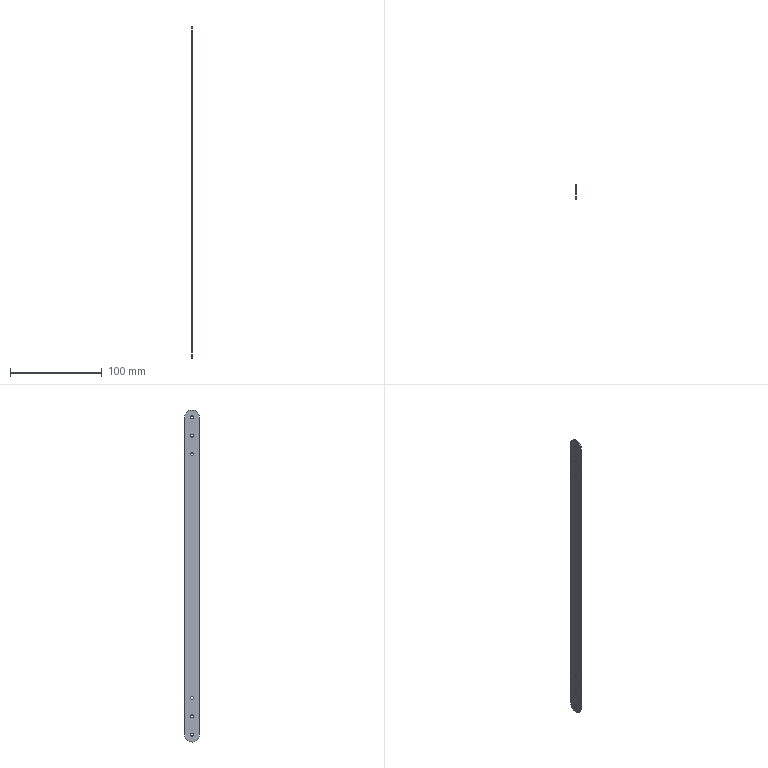Part | SolidWorks | features BaseBody 1 | 1 solid | 19 faces | box 1 x 16 x 361 mm | volume 5673 mm3 | cylinder 15 | plane 4 | commonest cylinder face diameters 3.2 x12 16 x3
STEP:
#1=CARTESIAN_POINT('',(1.,0.,-232.464));
#2=VERTEX_POINT('',#1);
#3=CARTESIAN_POINT('',(1.,0.,-235.664));
#4=VERTEX_POINT('',#3);
#5=CARTESIAN_POINT('',(1.,0.,-234.064));
#6=DIRECTION('',(1.,0.,0.));
#7=DIRECTION('',(0.,0.,1.));
#8=AXIS2_PLACEMENT_3D('',#5,#6,#7);
#9=CIRCLE('',#8,1.6);
#10=EDGE_CURVE('',#2,#4,#9,.T.);
#11=ORIENTED_EDGE('',*,*,#10,.T.);
#12=CARTESIAN_POINT('',(0.,0.,-235.664));
#13=VERTEX_POINT('',#12);
#14=CARTESIAN_POINT('',(1.,0.,-235.664));
#15=DIRECTION('',(-1.,0.,0.));
#16=VECTOR('',#15,1000.);
#17=LINE('',#14,#16);
#18=EDGE_CURVE('',#4,#13,#17,.T.);
#19=ORIENTED_EDGE('',*,*,#18,.T.);
#20=CARTESIAN_POINT('',(0.,0.,-232.464));
#21=VERTEX_POINT('',#20);
#22=CARTESIAN_POINT('',(0.,0.,-234.064));
#23=DIRECTION('',(-1.,0.,0.));
#24=DIRECTION('',(0.,0.,1.));
#25=AXIS2_PLACEMENT_3D('',#22,#23,#24);
#26=CIRCLE('',#25,1.6);
#27=EDGE_CURVE('',#13,#21,#26,.T.);
#28=ORIENTED_EDGE('',*,*,#27,.T.);
#29=CARTESIAN_POINT('',(1.,0.,-232.464));
#30=DIRECTION('',(-1.,0.,0.));
#31=VECTOR('',#30,1000.);
#32=LINE('',#29,#31);
#33=EDGE_CURVE('',#2,#21,#32,.T.);
#34=ORIENTED_EDGE('',*,*,#33,.F.);
#35=EDGE_LOOP('',(#11,#19,#28,#34));
#36=FACE_OUTER_BOUND('',#35,.T.);
#37=CARTESIAN_POINT('',(1.,0.,-234.064));
#38=DIRECTION('',(-1.,0.,0.));
#39=DIRECTION('',(0.,0.,1.));
#40=AXIS2_PLACEMENT_3D('',#37,#38,#39);
#41=CYLINDRICAL_SURFACE('',#40,1.6);
#42=ADVANCED_FACE('',(#36),#41,.F.);
#43=CARTESIAN_POINT('',(1.,0.,-275.664));
#44=VERTEX_POINT('',#43);
#45=CARTESIAN_POINT('',(1.,0.,-272.464));
#46=VERTEX_POINT('',#45);
#47=CARTESIAN_POINT('',(1.,0.,-274.064));
#48=DIRECTION('',(-1.,0.,0.));
#49=DIRECTION('',(0.,0.,1.));
#50=AXIS2_PLACEMENT_3D('',#47,#48,#49);
#51=CIRCLE('',#50,1.6);
#52=EDGE_CURVE('',#44,#46,#51,.T.);
#53=ORIENTED_EDGE('',*,*,#52,.F.);
#54=CARTESIAN_POINT('',(0.,0.,-275.664));
#55=VERTEX_POINT('',#54);
#56=CARTESIAN_POINT('',(1.,0.,-275.664));
#57=DIRECTION('',(-1.,0.,0.));
#58=VECTOR('',#57,1000.);
#59=LINE('',#56,#58);
#60=EDGE_CURVE('',#44,#55,#59,.T.);
#61=ORIENTED_EDGE('',*,*,#60,.T.);
#62=CARTESIAN_POINT('',(0.,0.,-272.464));
#63=VERTEX_POINT('',#62);
#64=CARTESIAN_POINT('',(0.,0.,-274.064));
#65=DIRECTION('',(-1.,0.,0.));
#66=DIRECTION('',(0.,0.,1.));
#67=AXIS2_PLACEMENT_3D('',#64,#65,#66);
#68=CIRCLE('',#67,1.6);
#69=EDGE_CURVE('',#55,#63,#68,.T.);
#70=ORIENTED_EDGE('',*,*,#69,.T.);
#71=CARTESIAN_POINT('',(1.,0.,-272.464));
#72=DIRECTION('',(-1.,0.,0.));
#73=VECTOR('',#72,1000.);
#74=LINE('',#71,#73);
#75=EDGE_CURVE('',#46,#63,#74,.T.);
#76=ORIENTED_EDGE('',*,*,#75,.F.);
#77=EDGE_LOOP('',(#53,#61,#70,#76));
#78=FACE_OUTER_BOUND('',#77,.T.);
#79=CARTESIAN_POINT('',(1.,0.,-274.064));
#80=DIRECTION('',(-1.,0.,0.));
#81=DIRECTION('',(0.,0.,1.));
#82=AXIS2_PLACEMENT_3D('',#79,#80,#81);
#83=CYLINDRICAL_SURFACE('',#82,1.6);
#84=ADVANCED_FACE('',(#78),#83,.F.);
#85=CARTESIAN_POINT('',(1.,0.,49.336));
#86=VERTEX_POINT('',#85);
#87=CARTESIAN_POINT('',(1.,0.,52.536));
#88=VERTEX_POINT('',#87);
#89=CARTESIAN_POINT('',(1.,0.,50.936));
#90=DIRECTION('',(-1.,0.,0.));
#91=DIRECTION('',(0.,0.,1.));
#92=AXIS2_PLACEMENT_3D('',#89,#90,#91);
#93=CIRCLE('',#92,1.6);
#94=EDGE_CURVE('',#86,#88,#93,.T.);
#95=ORIENTED_EDGE('',*,*,#94,.F.);
#96=CARTESIAN_POINT('',(0.,0.,49.336));
#97=VERTEX_POINT('',#96);
#98=CARTESIAN_POINT('',(1.,0.,49.336));
#99=DIRECTION('',(-1.,0.,0.));
#100=VECTOR('',#99,1000.);
#101=LINE('',#98,#100);
#102=EDGE_CURVE('',#86,#97,#101,.T.);
#103=ORIENTED_EDGE('',*,*,#102,.T.);
#104=CARTESIAN_POINT('',(0.,0.,52.536));
#105=VERTEX_POINT('',#104);
#106=CARTESIAN_POINT('',(0.,0.,50.936));
#107=DIRECTION('',(-1.,0.,0.));
#108=DIRECTION('',(0.,0.,1.));
#109=AXIS2_PLACEMENT_3D('',#106,#107,#108);
#110=CIRCLE('',#109,1.6);
#111=EDGE_CURVE('',#97,#105,#110,.T.);
#112=ORIENTED_EDGE('',*,*,#111,.T.);
#113=CARTESIAN_POINT('',(1.,0.,52.536));
#114=DIRECTION('',(-1.,0.,0.));
#115=VECTOR('',#114,1000.);
#116=LINE('',#113,#115);
#117=EDGE_CURVE('',#88,#105,#116,.T.);
#118=ORIENTED_EDGE('',*,*,#117,.F.);
#119=EDGE_LOOP('',(#95,#103,#112,#118));
#120=FACE_OUTER_BOUND('',#119,.T.);
#121=CARTESIAN_POINT('',(1.,0.,50.936));
#122=DIRECTION('',(-1.,0.,0.));
#123=DIRECTION('',(0.,0.,1.));
#124=AXIS2_PLACEMENT_3D('',#121,#122,#123);
#125=CYLINDRICAL_SURFACE('',#124,1.6);
#126=ADVANCED_FACE('',(#120),#125,.F.);
#127=CARTESIAN_POINT('',(1.,0.,69.336));
#128=VERTEX_POINT('',#127);
#129=CARTESIAN_POINT('',(1.,0.,72.536));
#130=VERTEX_POINT('',#129);
#131=CARTESIAN_POINT('',(1.,0.,70.936));
#132=DIRECTION('',(-1.,0.,0.));
#133=DIRECTION('',(0.,0.,1.));
#134=AXIS2_PLACEMENT_3D('',#131,#132,#133);
#135=CIRCLE('',#134,1.6);
#136=EDGE_CURVE('',#128,#130,#135,.T.);
#137=ORIENTED_EDGE('',*,*,#136,.F.);
#138=CARTESIAN_POINT('',(0.,0.,69.336));
#139=VERTEX_POINT('',#138);
#140=CARTESIAN_POINT('',(1.,0.,69.336));
#141=DIRECTION('',(-1.,0.,0.));
#142=VECTOR('',#141,1000.);
#143=LINE('',#140,#142);
#144=EDGE_CURVE('',#128,#139,#143,.T.);
#145=ORIENTED_EDGE('',*,*,#144,.T.);
#146=CARTESIAN_POINT('',(0.,0.,72.536));
#147=VERTEX_POINT('',#146);
#148=CARTESIAN_POINT('',(0.,0.,70.936));
#149=DIRECTION('',(-1.,0.,0.));
#150=DIRECTION('',(0.,0.,1.));
#151=AXIS2_PLACEMENT_3D('',#148,#149,#150);
#152=CIRCLE('',#151,1.6);
#153=EDGE_CURVE('',#139,#147,#152,.T.);
#154=ORIENTED_EDGE('',*,*,#153,.T.);
#155=CARTESIAN_POINT('',(1.,0.,72.536));
#156=DIRECTION('',(-1.,0.,0.));
#157=VECTOR('',#156,1000.);
#158=LINE('',#155,#157);
#159=EDGE_CURVE('',#130,#147,#158,.T.);
#160=ORIENTED_EDGE('',*,*,#159,.F.);
#161=EDGE_LOOP('',(#137,#145,#154,#160));
#162=FACE_OUTER_BOUND('',#161,.T.);
#163=CARTESIAN_POINT('',(1.,0.,70.936));
#164=DIRECTION('',(-1.,0.,0.));
#165=DIRECTION('',(0.,0.,1.));
#166=AXIS2_PLACEMENT_3D('',#163,#164,#165);
#167=CYLINDRICAL_SURFACE('',#166,1.6);
#168=ADVANCED_FACE('',(#162),#167,.F.);
#169=CARTESIAN_POINT('',(1.,0.,29.336));
#170=VERTEX_POINT('',#169);
#171=CARTESIAN_POINT('',(1.,0.,32.536));
#172=VERTEX_POINT('',#171);
#173=CARTESIAN_POINT('',(1.,0.,30.936));
#174=DIRECTION('',(-1.,0.,0.));
#175=DIRECTION('',(0.,0.,1.));
#176=AXIS2_PLACEMENT_3D('',#173,#174,#175);
#177=CIRCLE('',#176,1.6);
#178=EDGE_CURVE('',#170,#172,#177,.T.);
#179=ORIENTED_EDGE('',*,*,#178,.F.);
#180=CARTESIAN_POINT('',(0.,0.,29.336));
#181=VERTEX_POINT('',#180);
#182=CARTESIAN_POINT('',(1.,0.,29.336));
#183=DIRECTION('',(-1.,0.,0.));
#184=VECTOR('',#183,1000.);
#185=LINE('',#182,#184);
#186=EDGE_CURVE('',#170,#181,#185,.T.);
#187=ORIENTED_EDGE('',*,*,#186,.T.);
#188=CARTESIAN_POINT('',(0.,0.,32.536));
#189=VERTEX_POINT('',#188);
#190=CARTESIAN_POINT('',(0.,0.,30.936));
#191=DIRECTION('',(-1.,0.,0.));
#192=DIRECTION('',(0.,0.,1.));
#193=AXIS2_PLACEMENT_3D('',#190,#191,#192);
#194=CIRCLE('',#193,1.6);
#195=EDGE_CURVE('',#181,#189,#194,.T.);
#196=ORIENTED_EDGE('',*,*,#195,.T.);
#197=CARTESIAN_POINT('',(1.,0.,32.536));
#198=DIRECTION('',(-1.,0.,0.));
#199=VECTOR('',#198,1000.);
#200=LINE('',#197,#199);
#201=EDGE_CURVE('',#172,#189,#200,.T.);
#202=ORIENTED_EDGE('',*,*,#201,.F.);
#203=EDGE_LOOP('',(#179,#187,#196,#202));
#204=FACE_OUTER_BOUND('',#203,.T.);
#205=CARTESIAN_POINT('',(1.,0.,30.936));
#206=DIRECTION('',(-1.,0.,0.));
#207=DIRECTION('',(0.,0.,1.));
#208=AXIS2_PLACEMENT_3D('',#205,#206,#207);
#209=CYLINDRICAL_SURFACE('',#208,1.6);
#210=ADVANCED_FACE('',(#204),#209,.F.);
#211=CARTESIAN_POINT('',(1.,0.,-255.664));
#212=VERTEX_POINT('',#211);
#213=CARTESIAN_POINT('',(1.,0.,-252.464));
#214=VERTEX_POINT('',#213);
#215=CARTESIAN_POINT('',(1.,0.,-254.064));
#216=DIRECTION('',(-1.,0.,0.));
#217=DIRECTION('',(0.,0.,1.));
#218=AXIS2_PLACEMENT_3D('',#215,#216,#217);
#219=CIRCLE('',#218,1.6);
#220=EDGE_CURVE('',#212,#214,#219,.T.);
#221=ORIENTED_EDGE('',*,*,#220,.F.);
#222=CARTESIAN_POINT('',(0.,0.,-255.664));
#223=VERTEX_POINT('',#222);
#224=CARTESIAN_POINT('',(1.,0.,-255.664));
#225=DIRECTION('',(-1.,0.,0.));
#226=VECTOR('',#225,1000.);
#227=LINE('',#224,#226);
#228=EDGE_CURVE('',#212,#223,#227,.T.);
#229=ORIENTED_EDGE('',*,*,#228,.T.);
#230=CARTESIAN_POINT('',(0.,0.,-252.464));
#231=VERTEX_POINT('',#230);
#232=CARTESIAN_POINT('',(0.,0.,-254.064));
#233=DIRECTION('',(-1.,0.,0.));
#234=DIRECTION('',(0.,0.,1.));
#235=AXIS2_PLACEMENT_3D('',#232,#233,#234);
#236=CIRCLE('',#235,1.6);
#237=EDGE_CURVE('',#223,#231,#236,.T.);
#238=ORIENTED_EDGE('',*,*,#237,.T.);
#239=CARTESIAN_POINT('',(1.,0.,-252.464));
#240=DIRECTION('',(-1.,0.,0.));
#241=VECTOR('',#240,1000.);
#242=LINE('',#239,#241);
#243=EDGE_CURVE('',#214,#231,#242,.T.);
#244=ORIENTED_EDGE('',*,*,#243,.F.);
#245=EDGE_LOOP('',(#221,#229,#238,#244));
#246=FACE_OUTER_BOUND('',#245,.T.);
#247=CARTESIAN_POINT('',(1.,0.,-254.064));
#248=DIRECTION('',(-1.,0.,0.));
#249=DIRECTION('',(0.,0.,1.));
#250=AXIS2_PLACEMENT_3D('',#247,#248,#249);
#251=CYLINDRICAL_SURFACE('',#250,1.6);
#252=ADVANCED_FACE('',(#246),#251,.F.);
#253=CARTESIAN_POINT('',(1.,0.,78.936));
#254=VERTEX_POINT('',#253);
#255=CARTESIAN_POINT('',(1.,-8.,70.936));
#256=VERTEX_POINT('',#255);
#257=CARTESIAN_POINT('',(1.,0.,70.936));
#258=DIRECTION('',(1.,0.,0.));
#259=DIRECTION('',(0.,0.,1.));
#260=AXIS2_PLACEMENT_3D('',#257,#258,#259);
#261=CIRCLE('',#260,8.);
#262=EDGE_CURVE('',#254,#256,#261,.T.);
#263=ORIENTED_EDGE('',*,*,#262,.F.);
#264=CARTESIAN_POINT('',(0.,0.,78.936));
#265=VERTEX_POINT('',#264);
#266=CARTESIAN_POINT('',(1.,0.,78.936));
#267=DIRECTION('',(-1.,0.,0.));
#268=VECTOR('',#267,1000.);
#269=LINE('',#266,#268);
#270=EDGE_CURVE('',#254,#265,#269,.T.);
#271=ORIENTED_EDGE('',*,*,#270,.T.);
#272=CARTESIAN_POINT('',(0.,-8.,70.936));
#273=VERTEX_POINT('',#272);
#274=CARTESIAN_POINT('',(0.,0.,70.936));
#275=DIRECTION('',(1.,0.,0.));
#276=DIRECTION('',(0.,0.,1.));
#277=AXIS2_PLACEMENT_3D('',#274,#275,#276);
#278=CIRCLE('',#277,8.);
#279=EDGE_CURVE('',#265,#273,#278,.T.);
#280=ORIENTED_EDGE('',*,*,#279,.T.);
#281=CARTESIAN_POINT('',(0.5,-8.,70.936));
#282=DIRECTION('',(1.,0.,0.));
#283=VECTOR('',#282,1000.);
#284=LINE('',#281,#283);
#285=EDGE_CURVE('',#273,#256,#284,.T.);
#286=ORIENTED_EDGE('',*,*,#285,.T.);
#287=EDGE_LOOP('',(#263,#271,#280,#286));
#288=FACE_OUTER_BOUND('',#287,.T.);
#289=CARTESIAN_POINT('',(1.,0.,70.936));
#290=DIRECTION('',(-1.,0.,0.));
#291=DIRECTION('',(0.,0.,1.));
#292=AXIS2_PLACEMENT_3D('',#289,#290,#291);
#293=CYLINDRICAL_SURFACE('',#292,8.);
#294=ADVANCED_FACE('',(#288),#293,.T.);
#295=ORIENTED_EDGE('',*,*,#18,.F.);
#296=CARTESIAN_POINT('',(1.,0.,-234.064));
#297=DIRECTION('',(1.,0.,0.));
#298=DIRECTION('',(0.,0.,1.));
#299=AXIS2_PLACEMENT_3D('',#296,#297,#298);
#300=CIRCLE('',#299,1.6);
#301=EDGE_CURVE('',#4,#2,#300,.T.);
#302=ORIENTED_EDGE('',*,*,#301,.T.);
#303=ORIENTED_EDGE('',*,*,#33,.T.);
#304=CARTESIAN_POINT('',(0.,0.,-234.064));
#305=DIRECTION('',(-1.,0.,0.));
#306=DIRECTION('',(0.,0.,1.));
#307=AXIS2_PLACEMENT_3D('',#304,#305,#306);
#308=CIRCLE('',#307,1.6);
#309=EDGE_CURVE('',#21,#13,#308,.T.);
#310=ORIENTED_EDGE('',*,*,#309,.T.);
#311=EDGE_LOOP('',(#295,#302,#303,#310));
#312=FACE_OUTER_BOUND('',#311,.T.);
#313=CARTESIAN_POINT('',(1.,0.,-234.064));
#314=DIRECTION('',(-1.,0.,0.));
#315=DIRECTION('',(0.,0.,1.));
#316=AXIS2_PLACEMENT_3D('',#313,#314,#315);
#317=CYLINDRICAL_SURFACE('',#316,1.6);
#318=ADVANCED_FACE('',(#312),#317,.F.);
#319=ORIENTED_EDGE('',*,*,#309,.F.);
#320=ORIENTED_EDGE('',*,*,#27,.F.);
#321=EDGE_LOOP('',(#319,#320));
#322=FACE_BOUND('',#321,.T.);
#323=CARTESIAN_POINT('',(0.,0.,-274.064));
#324=DIRECTION('',(-1.,0.,0.));
#325=DIRECTION('',(0.,0.,1.));
#326=AXIS2_PLACEMENT_3D('',#323,#324,#325);
#327=CIRCLE('',#326,1.6);
#328=EDGE_CURVE('',#63,#55,#327,.T.);
#329=ORIENTED_EDGE('',*,*,#328,.F.);
#330=ORIENTED_EDGE('',*,*,#69,.F.);
#331=EDGE_LOOP('',(#329,#330));
#332=FACE_BOUND('',#331,.T.);
#333=CARTESIAN_POINT('',(0.,0.,50.936));
#334=DIRECTION('',(-1.,0.,0.));
#335=DIRECTION('',(0.,0.,1.));
#336=AXIS2_PLACEMENT_3D('',#333,#334,#335);
#337=CIRCLE('',#336,1.6);
#338=EDGE_CURVE('',#105,#97,#337,.T.);
#339=ORIENTED_EDGE('',*,*,#338,.F.);
#340=ORIENTED_EDGE('',*,*,#111,.F.);
#341=EDGE_LOOP('',(#339,#340));
#342=FACE_BOUND('',#341,.T.);
#343=CARTESIAN_POINT('',(0.,0.,70.936));
#344=DIRECTION('',(-1.,0.,0.));
#345=DIRECTION('',(0.,0.,1.));
#346=AXIS2_PLACEMENT_3D('',#343,#344,#345);
#347=CIRCLE('',#346,1.6);
#348=EDGE_CURVE('',#147,#139,#347,.T.);
#349=ORIENTED_EDGE('',*,*,#348,.F.);
#350=ORIENTED_EDGE('',*,*,#153,.F.);
#351=EDGE_LOOP('',(#349,#350));
#352=FACE_BOUND('',#351,.T.);
#353=CARTESIAN_POINT('',(0.,0.,30.936));
#354=DIRECTION('',(-1.,0.,0.));
#355=DIRECTION('',(0.,0.,1.));
#356=AXIS2_PLACEMENT_3D('',#353,#354,#355);
#357=CIRCLE('',#356,1.6);
#358=EDGE_CURVE('',#189,#181,#357,.T.);
#359=ORIENTED_EDGE('',*,*,#358,.F.);
#360=ORIENTED_EDGE('',*,*,#195,.F.);
#361=EDGE_LOOP('',(#359,#360));
#362=FACE_BOUND('',#361,.T.);
#363=CARTESIAN_POINT('',(0.,0.,-254.064));
#364=DIRECTION('',(-1.,0.,0.));
#365=DIRECTION('',(0.,0.,1.));
#366=AXIS2_PLACEMENT_3D('',#363,#364,#365);
#367=CIRCLE('',#366,1.6);
#368=EDGE_CURVE('',#231,#223,#367,.T.);
#369=ORIENTED_EDGE('',*,*,#368,.F.);
#370=ORIENTED_EDGE('',*,*,#237,.F.);
#371=EDGE_LOOP('',(#369,#370));
#372=FACE_BOUND('',#371,.T.);
#373=CARTESIAN_POINT('',(0.,8.,-274.064));
#374=VERTEX_POINT('',#373);
#375=CARTESIAN_POINT('',(0.,8.,70.936));
#376=VERTEX_POINT('',#375);
#377=CARTESIAN_POINT('',(0.,8.,-101.564));
#378=DIRECTION('',(0.,0.,1.));
#379=VECTOR('',#378,1000.);
#380=LINE('',#377,#379);
#381=EDGE_CURVE('',#374,#376,#380,.T.);
#382=ORIENTED_EDGE('',*,*,#381,.F.);
#383=CARTESIAN_POINT('',(0.,-8.,-274.064));
#384=VERTEX_POINT('',#383);
#385=CARTESIAN_POINT('',(0.,0.,-274.064));
#386=DIRECTION('',(1.,0.,0.));
#387=DIRECTION('',(0.,0.,1.));
#388=AXIS2_PLACEMENT_3D('',#385,#386,#387);
#389=CIRCLE('',#388,8.);
#390=EDGE_CURVE('',#384,#374,#389,.T.);
#391=ORIENTED_EDGE('',*,*,#390,.F.);
#392=CARTESIAN_POINT('',(0.,-8.,-101.564));
#393=DIRECTION('',(0.,0.,-1.));
#394=VECTOR('',#393,1000.);
#395=LINE('',#392,#394);
#396=EDGE_CURVE('',#273,#384,#395,.T.);
#397=ORIENTED_EDGE('',*,*,#396,.F.);
#398=ORIENTED_EDGE('',*,*,#279,.F.);
#399=CARTESIAN_POINT('',(0.,0.,70.936));
#400=DIRECTION('',(1.,0.,0.));
#401=DIRECTION('',(0.,0.,1.));
#402=AXIS2_PLACEMENT_3D('',#399,#400,#401);
#403=CIRCLE('',#402,8.);
#404=EDGE_CURVE('',#376,#265,#403,.T.);
#405=ORIENTED_EDGE('',*,*,#404,.F.);
#406=EDGE_LOOP('',(#382,#391,#397,#398,#405));
#407=FACE_OUTER_BOUND('',#406,.T.);
#408=CARTESIAN_POINT('',(0.,-8.,81.102));
#409=DIRECTION('',(1.,0.,0.));
#410=DIRECTION('',(0.,0.,-1.));
#411=AXIS2_PLACEMENT_3D('',#408,#409,#410);
#412=PLANE('',#411);
#413=ADVANCED_FACE('',(#322,#332,#342,#352,#362,#372,#407),#412,.F.);
#414=ORIENTED_EDGE('',*,*,#10,.F.);
#415=ORIENTED_EDGE('',*,*,#301,.F.);
#416=EDGE_LOOP('',(#414,#415));
#417=FACE_BOUND('',#416,.T.);
#418=CARTESIAN_POINT('',(1.,0.,-274.064));
#419=DIRECTION('',(-1.,0.,0.));
#420=DIRECTION('',(0.,0.,1.));
#421=AXIS2_PLACEMENT_3D('',#418,#419,#420);
#422=CIRCLE('',#421,1.6);
#423=EDGE_CURVE('',#46,#44,#422,.T.);
#424=ORIENTED_EDGE('',*,*,#423,.T.);
#425=ORIENTED_EDGE('',*,*,#52,.T.);
#426=EDGE_LOOP('',(#424,#425));
#427=FACE_BOUND('',#426,.T.);
#428=CARTESIAN_POINT('',(1.,0.,50.936));
#429=DIRECTION('',(-1.,0.,0.));
#430=DIRECTION('',(0.,0.,1.));
#431=AXIS2_PLACEMENT_3D('',#428,#429,#430);
#432=CIRCLE('',#431,1.6);
#433=EDGE_CURVE('',#88,#86,#432,.T.);
#434=ORIENTED_EDGE('',*,*,#433,.T.);
#435=ORIENTED_EDGE('',*,*,#94,.T.);
#436=EDGE_LOOP('',(#434,#435));
#437=FACE_BOUND('',#436,.T.);
#438=CARTESIAN_POINT('',(1.,0.,70.936));
#439=DIRECTION('',(-1.,0.,0.));
#440=DIRECTION('',(0.,0.,1.));
#441=AXIS2_PLACEMENT_3D('',#438,#439,#440);
#442=CIRCLE('',#441,1.6);
#443=EDGE_CURVE('',#130,#128,#442,.T.);
#444=ORIENTED_EDGE('',*,*,#443,.T.);
#445=ORIENTED_EDGE('',*,*,#136,.T.);
#446=EDGE_LOOP('',(#444,#445));
#447=FACE_BOUND('',#446,.T.);
#448=CARTESIAN_POINT('',(1.,0.,30.936));
#449=DIRECTION('',(-1.,0.,0.));
#450=DIRECTION('',(0.,0.,1.));
#451=AXIS2_PLACEMENT_3D('',#448,#449,#450);
#452=CIRCLE('',#451,1.6);
#453=EDGE_CURVE('',#172,#170,#452,.T.);
#454=ORIENTED_EDGE('',*,*,#453,.T.);
#455=ORIENTED_EDGE('',*,*,#178,.T.);
#456=EDGE_LOOP('',(#454,#455));
#457=FACE_BOUND('',#456,.T.);
#458=CARTESIAN_POINT('',(1.,0.,-254.064));
#459=DIRECTION('',(-1.,0.,0.));
#460=DIRECTION('',(0.,0.,1.));
#461=AXIS2_PLACEMENT_3D('',#458,#459,#460);
#462=CIRCLE('',#461,1.6);
#463=EDGE_CURVE('',#214,#212,#462,.T.);
#464=ORIENTED_EDGE('',*,*,#463,.T.);
#465=ORIENTED_EDGE('',*,*,#220,.T.);
#466=EDGE_LOOP('',(#464,#465));
#467=FACE_BOUND('',#466,.T.);
#468=CARTESIAN_POINT('',(1.,-8.,-274.064));
#469=VERTEX_POINT('',#468);
#470=CARTESIAN_POINT('',(1.,8.,-274.064));
#471=VERTEX_POINT('',#470);
#472=CARTESIAN_POINT('',(1.,0.,-274.064));
#473=DIRECTION('',(1.,0.,0.));
#474=DIRECTION('',(0.,0.,1.));
#475=AXIS2_PLACEMENT_3D('',#472,#473,#474);
#476=CIRCLE('',#475,8.);
#477=EDGE_CURVE('',#469,#471,#476,.T.);
#478=ORIENTED_EDGE('',*,*,#477,.T.);
#479=CARTESIAN_POINT('',(1.,8.,70.936));
#480=VERTEX_POINT('',#479);
#481=CARTESIAN_POINT('',(1.,8.,-101.564));
#482=DIRECTION('',(0.,0.,1.));
#483=VECTOR('',#482,1000.);
#484=LINE('',#481,#483);
#485=EDGE_CURVE('',#471,#480,#484,.T.);
#486=ORIENTED_EDGE('',*,*,#485,.T.);
#487=CARTESIAN_POINT('',(1.,0.,70.936));
#488=DIRECTION('',(1.,0.,0.));
#489=DIRECTION('',(0.,0.,1.));
#490=AXIS2_PLACEMENT_3D('',#487,#488,#489);
#491=CIRCLE('',#490,8.);
#492=EDGE_CURVE('',#480,#254,#491,.T.);
#493=ORIENTED_EDGE('',*,*,#492,.T.);
#494=ORIENTED_EDGE('',*,*,#262,.T.);
#495=CARTESIAN_POINT('',(1.,-8.,-101.564));
#496=DIRECTION('',(0.,0.,-1.));
#497=VECTOR('',#496,1000.);
#498=LINE('',#495,#497);
#499=EDGE_CURVE('',#256,#469,#498,.T.);
#500=ORIENTED_EDGE('',*,*,#499,.T.);
#501=EDGE_LOOP('',(#478,#486,#493,#494,#500));
#502=FACE_OUTER_BOUND('',#501,.T.);
#503=CARTESIAN_POINT('',(1.,-8.,81.102));
#504=DIRECTION('',(1.,0.,0.));
#505=DIRECTION('',(0.,0.,-1.));
#506=AXIS2_PLACEMENT_3D('',#503,#504,#505);
#507=PLANE('',#506);
#508=ADVANCED_FACE('',(#417,#427,#437,#447,#457,#467,#502),#507,.T.);
#509=ORIENTED_EDGE('',*,*,#60,.F.);
#510=ORIENTED_EDGE('',*,*,#423,.F.);
#511=ORIENTED_EDGE('',*,*,#75,.T.);
#512=ORIENTED_EDGE('',*,*,#328,.T.);
#513=EDGE_LOOP('',(#509,#510,#511,#512));
#514=FACE_OUTER_BOUND('',#513,.T.);
#515=CARTESIAN_POINT('',(1.,0.,-274.064));
#516=DIRECTION('',(-1.,0.,0.));
#517=DIRECTION('',(0.,0.,1.));
#518=AXIS2_PLACEMENT_3D('',#515,#516,#517);
#519=CYLINDRICAL_SURFACE('',#518,1.6);
#520=ADVANCED_FACE('',(#514),#519,.F.);
#521=ORIENTED_EDGE('',*,*,#102,.F.);
#522=ORIENTED_EDGE('',*,*,#433,.F.);
#523=ORIENTED_EDGE('',*,*,#117,.T.);
#524=ORIENTED_EDGE('',*,*,#338,.T.);
#525=EDGE_LOOP('',(#521,#522,#523,#524));
#526=FACE_OUTER_BOUND('',#525,.T.);
#527=CARTESIAN_POINT('',(1.,0.,50.936));
#528=DIRECTION('',(-1.,0.,0.));
#529=DIRECTION('',(0.,0.,1.));
#530=AXIS2_PLACEMENT_3D('',#527,#528,#529);
#531=CYLINDRICAL_SURFACE('',#530,1.6);
#532=ADVANCED_FACE('',(#526),#531,.F.);
#533=ORIENTED_EDGE('',*,*,#144,.F.);
#534=ORIENTED_EDGE('',*,*,#443,.F.);
#535=ORIENTED_EDGE('',*,*,#159,.T.);
#536=ORIENTED_EDGE('',*,*,#348,.T.);
#537=EDGE_LOOP('',(#533,#534,#535,#536));
#538=FACE_OUTER_BOUND('',#537,.T.);
#539=CARTESIAN_POINT('',(1.,0.,70.936));
#540=DIRECTION('',(-1.,0.,0.));
#541=DIRECTION('',(0.,0.,1.));
#542=AXIS2_PLACEMENT_3D('',#539,#540,#541);
#543=CYLINDRICAL_SURFACE('',#542,1.6);
#544=ADVANCED_FACE('',(#538),#543,.F.);
#545=ORIENTED_EDGE('',*,*,#186,.F.);
#546=ORIENTED_EDGE('',*,*,#453,.F.);
#547=ORIENTED_EDGE('',*,*,#201,.T.);
#548=ORIENTED_EDGE('',*,*,#358,.T.);
#549=EDGE_LOOP('',(#545,#546,#547,#548));
#550=FACE_OUTER_BOUND('',#549,.T.);
#551=CARTESIAN_POINT('',(1.,0.,30.936));
#552=DIRECTION('',(-1.,0.,0.));
#553=DIRECTION('',(0.,0.,1.));
#554=AXIS2_PLACEMENT_3D('',#551,#552,#553);
#555=CYLINDRICAL_SURFACE('',#554,1.6);
#556=ADVANCED_FACE('',(#550),#555,.F.);
#557=ORIENTED_EDGE('',*,*,#228,.F.);
#558=ORIENTED_EDGE('',*,*,#463,.F.);
#559=ORIENTED_EDGE('',*,*,#243,.T.);
#560=ORIENTED_EDGE('',*,*,#368,.T.);
#561=EDGE_LOOP('',(#557,#558,#559,#560));
#562=FACE_OUTER_BOUND('',#561,.T.);
#563=CARTESIAN_POINT('',(1.,0.,-254.064));
#564=DIRECTION('',(-1.,0.,0.));
#565=DIRECTION('',(0.,0.,1.));
#566=AXIS2_PLACEMENT_3D('',#563,#564,#565);
#567=CYLINDRICAL_SURFACE('',#566,1.6);
#568=ADVANCED_FACE('',(#562),#567,.F.);
#569=ORIENTED_EDGE('',*,*,#270,.F.);
#570=ORIENTED_EDGE('',*,*,#492,.F.);
#571=CARTESIAN_POINT('',(0.5,8.,70.936));
#572=DIRECTION('',(1.,0.,0.));
#573=VECTOR('',#572,1000.);
#574=LINE('',#571,#573);
#575=EDGE_CURVE('',#376,#480,#574,.T.);
#576=ORIENTED_EDGE('',*,*,#575,.F.);
#577=ORIENTED_EDGE('',*,*,#404,.T.);
#578=EDGE_LOOP('',(#569,#570,#576,#577));
#579=FACE_OUTER_BOUND('',#578,.T.);
#580=CARTESIAN_POINT('',(1.,0.,70.936));
#581=DIRECTION('',(-1.,0.,0.));
#582=DIRECTION('',(0.,0.,1.));
#583=AXIS2_PLACEMENT_3D('',#580,#581,#582);
#584=CYLINDRICAL_SURFACE('',#583,8.);
#585=ADVANCED_FACE('',(#579),#584,.T.);
#586=ORIENTED_EDGE('',*,*,#575,.T.);
#587=ORIENTED_EDGE('',*,*,#485,.F.);
#588=CARTESIAN_POINT('',(0.5,8.,-274.064));
#589=DIRECTION('',(1.,0.,0.));
#590=VECTOR('',#589,1000.);
#591=LINE('',#588,#590);
#592=EDGE_CURVE('',#374,#471,#591,.T.);
#593=ORIENTED_EDGE('',*,*,#592,.F.);
#594=ORIENTED_EDGE('',*,*,#381,.T.);
#595=EDGE_LOOP('',(#586,#587,#593,#594));
#596=FACE_OUTER_BOUND('',#595,.T.);
#597=CARTESIAN_POINT('',(0.,8.,70.936));
#598=DIRECTION('',(0.,-1.,0.));
#599=DIRECTION('',(0.,0.,-1.));
#600=AXIS2_PLACEMENT_3D('',#597,#598,#599);
#601=PLANE('',#600);
#602=ADVANCED_FACE('',(#596),#601,.F.);
#603=ORIENTED_EDGE('',*,*,#592,.T.);
#604=ORIENTED_EDGE('',*,*,#477,.F.);
#605=CARTESIAN_POINT('',(0.5,-8.,-274.064));
#606=DIRECTION('',(1.,0.,0.));
#607=VECTOR('',#606,1000.);
#608=LINE('',#605,#607);
#609=EDGE_CURVE('',#384,#469,#608,.T.);
#610=ORIENTED_EDGE('',*,*,#609,.F.);
#611=ORIENTED_EDGE('',*,*,#390,.T.);
#612=EDGE_LOOP('',(#603,#604,#610,#611));
#613=FACE_OUTER_BOUND('',#612,.T.);
#614=CARTESIAN_POINT('',(1.,0.,-274.064));
#615=DIRECTION('',(-1.,0.,0.));
#616=DIRECTION('',(0.,0.,1.));
#617=AXIS2_PLACEMENT_3D('',#614,#615,#616);
#618=CYLINDRICAL_SURFACE('',#617,8.);
#619=ADVANCED_FACE('',(#613),#618,.T.);
#620=ORIENTED_EDGE('',*,*,#609,.T.);
#621=ORIENTED_EDGE('',*,*,#499,.F.);
#622=ORIENTED_EDGE('',*,*,#285,.F.);
#623=ORIENTED_EDGE('',*,*,#396,.T.);
#624=EDGE_LOOP('',(#620,#621,#622,#623));
#625=FACE_OUTER_BOUND('',#624,.T.);
#626=CARTESIAN_POINT('',(0.,-8.,-274.064));
#627=DIRECTION('',(0.,1.,0.));
#628=DIRECTION('',(0.,0.,1.));
#629=AXIS2_PLACEMENT_3D('',#626,#627,#628);
#630=PLANE('',#629);
#631=ADVANCED_FACE('',(#625),#630,.F.);
#632=CLOSED_SHELL('',(#42,#84,#126,#168,#210,#252,#294,#318,#413,#508,#520,#532,#544,#556,#568,#585,#602,#619,#631));
#633=MANIFOLD_SOLID_BREP('',#632);
#634=CARTESIAN_POINT('',(0.,0.,0.));
#635=DIRECTION('',(0.,0.,1.));
#636=DIRECTION('',(1.,0.,0.));
#637=AXIS2_PLACEMENT_3D('',#634,#635,#636);
#638=(LENGTH_UNIT()NAMED_UNIT(*)SI_UNIT(.MILLI.,.METRE.));
#639=UNCERTAINTY_MEASURE_WITH_UNIT(LENGTH_MEASURE(0.00001),#638,'','');
#640=(NAMED_UNIT(*)PLANE_ANGLE_UNIT()SI_UNIT($,.RADIAN.));
#641=(NAMED_UNIT(*)SI_UNIT($,.STERADIAN.)SOLID_ANGLE_UNIT());
#642=(GEOMETRIC_REPRESENTATION_CONTEXT(3)GLOBAL_UNCERTAINTY_ASSIGNED_CONTEXT((#639))GLOBAL_UNIT_ASSIGNED_CONTEXT((#638,#640,#641))REPRESENTATION_CONTEXT('',''));
#643=ADVANCED_BREP_SHAPE_REPRESENTATION('',(#633,#637),#642);